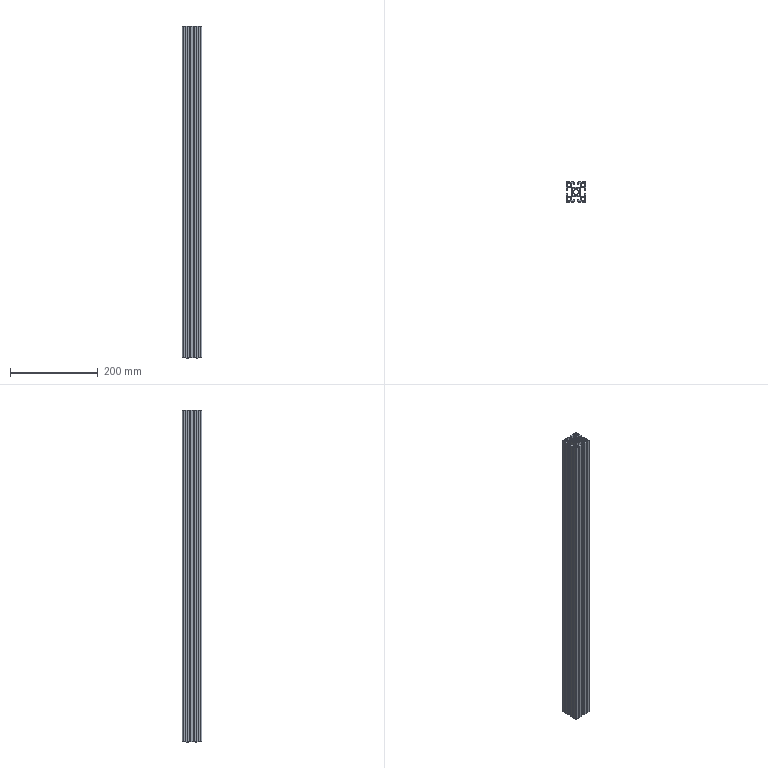Part | STEP file | 4545 Al PC rack upright | 1 solid | 262 faces | box 45 x 45 x 758.77 mm | volume 526470 mm3 | plane 186 | cylinder 76 | commonest cylinder face diameters 2 x44 8 x20 12 x8 4 x4